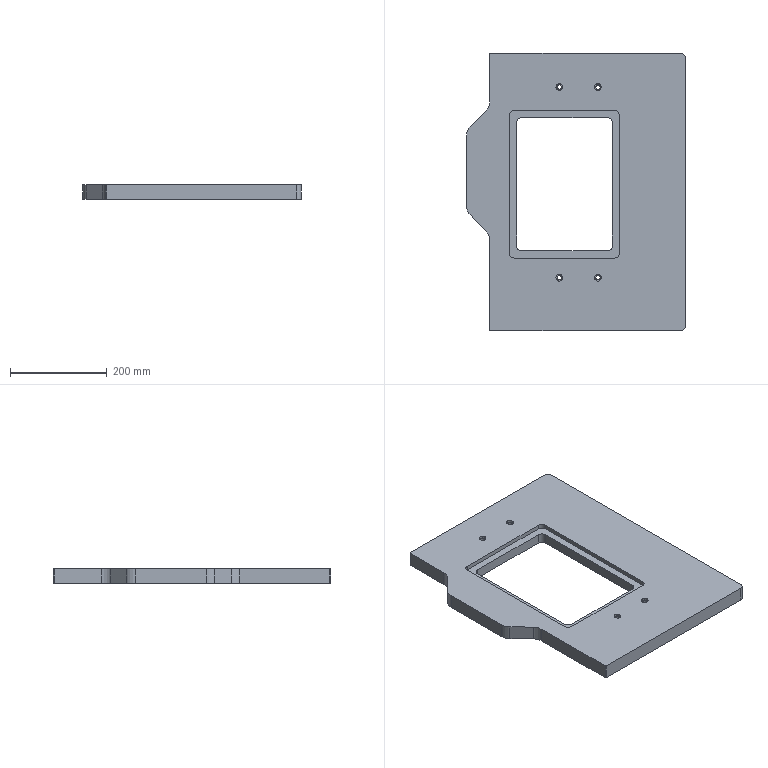Part | STEP file | Substructure | 1 solid | 47 faces | box 453 x 575 x 30 mm | volume 5515356 mm3 | cylinder 24 | plane 23 | commonest cylinder face diameters 20 x10 9 x4 14 x4 50 x4 4 x2